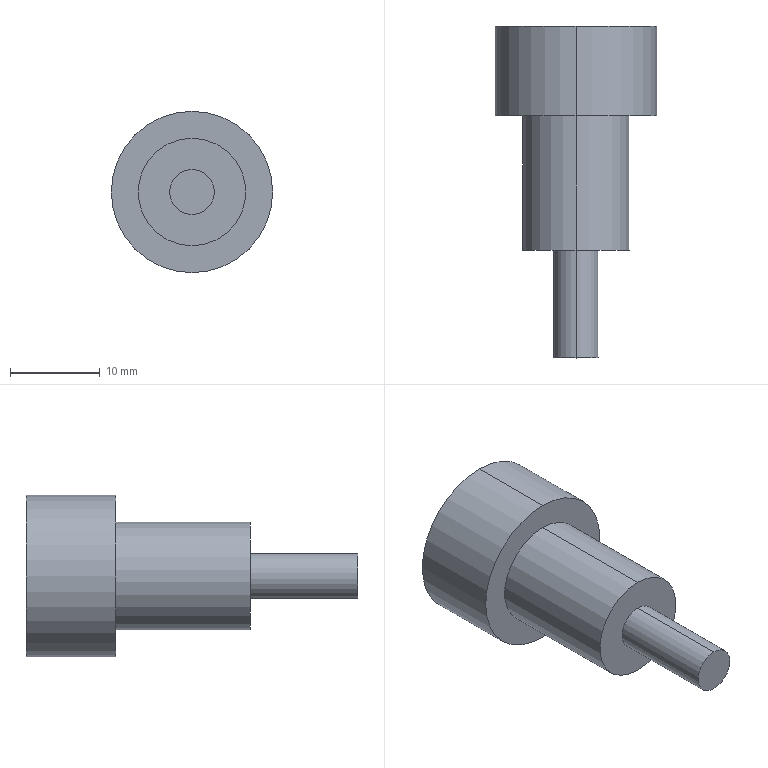Part | SolidWorks | features ICE 3, Extrusion 1 | 1 solid | 17 faces | box 18 x 37 x 18 mm | volume 4200 mm3 | plane 11 | cylinder 6 | commonest cylinder face diameters 5 x2 12 x2 18 x2
STEP:
#1=CARTESIAN_POINT('',(0.,37.,9.));
#2=VERTEX_POINT('',#1);
#3=CARTESIAN_POINT('',(0.,37.,-9.));
#4=VERTEX_POINT('',#3);
#5=CARTESIAN_POINT('',(0.,37.,0.));
#6=DIRECTION('',(0.,1.,0.));
#7=DIRECTION('',(0.,0.,1.));
#8=AXIS2_PLACEMENT_3D('',#5,#6,#7);
#9=CIRCLE('',#8,9.);
#10=EDGE_CURVE('',#2,#4,#9,.T.);
#11=ORIENTED_EDGE('',*,*,#10,.F.);
#12=CARTESIAN_POINT('',(0.,27.,9.));
#13=VERTEX_POINT('',#12);
#14=CARTESIAN_POINT('',(0.,37.,9.));
#15=DIRECTION('',(0.,-1.,0.));
#16=VECTOR('',#15,1000.);
#17=LINE('',#14,#16);
#18=EDGE_CURVE('',#2,#13,#17,.T.);
#19=ORIENTED_EDGE('',*,*,#18,.T.);
#20=CARTESIAN_POINT('',(0.,27.,-9.));
#21=VERTEX_POINT('',#20);
#22=CARTESIAN_POINT('',(0.,27.,0.));
#23=DIRECTION('',(0.,1.,0.));
#24=DIRECTION('',(0.,0.,1.));
#25=AXIS2_PLACEMENT_3D('',#22,#23,#24);
#26=CIRCLE('',#25,9.);
#27=EDGE_CURVE('',#13,#21,#26,.T.);
#28=ORIENTED_EDGE('',*,*,#27,.T.);
#29=CARTESIAN_POINT('',(0.,37.,-9.));
#30=DIRECTION('',(0.,-1.,0.));
#31=VECTOR('',#30,1000.);
#32=LINE('',#29,#31);
#33=EDGE_CURVE('',#4,#21,#32,.T.);
#34=ORIENTED_EDGE('',*,*,#33,.F.);
#35=EDGE_LOOP('',(#11,#19,#28,#34));
#36=FACE_OUTER_BOUND('',#35,.T.);
#37=CARTESIAN_POINT('',(0.,37.,0.));
#38=DIRECTION('',(0.,-1.,0.));
#39=DIRECTION('',(0.,0.,-1.));
#40=AXIS2_PLACEMENT_3D('',#37,#38,#39);
#41=CYLINDRICAL_SURFACE('',#40,9.);
#42=ADVANCED_FACE('',(#36),#41,.T.);
#43=CARTESIAN_POINT('',(0.,27.,6.));
#44=VERTEX_POINT('',#43);
#45=CARTESIAN_POINT('',(0.,27.,-6.));
#46=VERTEX_POINT('',#45);
#47=CARTESIAN_POINT('',(0.,27.,0.));
#48=DIRECTION('',(0.,1.,0.));
#49=DIRECTION('',(0.,0.,1.));
#50=AXIS2_PLACEMENT_3D('',#47,#48,#49);
#51=CIRCLE('',#50,6.);
#52=EDGE_CURVE('',#44,#46,#51,.T.);
#53=ORIENTED_EDGE('',*,*,#52,.F.);
#54=CARTESIAN_POINT('',(0.,12.,6.));
#55=VERTEX_POINT('',#54);
#56=CARTESIAN_POINT('',(0.,27.,6.));
#57=DIRECTION('',(0.,-1.,0.));
#58=VECTOR('',#57,1000.);
#59=LINE('',#56,#58);
#60=EDGE_CURVE('',#44,#55,#59,.T.);
#61=ORIENTED_EDGE('',*,*,#60,.T.);
#62=CARTESIAN_POINT('',(0.,12.,-6.));
#63=VERTEX_POINT('',#62);
#64=CARTESIAN_POINT('',(0.,12.,0.));
#65=DIRECTION('',(0.,1.,0.));
#66=DIRECTION('',(0.,0.,1.));
#67=AXIS2_PLACEMENT_3D('',#64,#65,#66);
#68=CIRCLE('',#67,6.);
#69=EDGE_CURVE('',#55,#63,#68,.T.);
#70=ORIENTED_EDGE('',*,*,#69,.T.);
#71=CARTESIAN_POINT('',(0.,27.,-6.));
#72=DIRECTION('',(0.,-1.,0.));
#73=VECTOR('',#72,1000.);
#74=LINE('',#71,#73);
#75=EDGE_CURVE('',#46,#63,#74,.T.);
#76=ORIENTED_EDGE('',*,*,#75,.F.);
#77=EDGE_LOOP('',(#53,#61,#70,#76));
#78=FACE_OUTER_BOUND('',#77,.T.);
#79=CARTESIAN_POINT('',(0.,27.,0.));
#80=DIRECTION('',(0.,-1.,0.));
#81=DIRECTION('',(0.,0.,-1.));
#82=AXIS2_PLACEMENT_3D('',#79,#80,#81);
#83=CYLINDRICAL_SURFACE('',#82,6.);
#84=ADVANCED_FACE('',(#78),#83,.T.);
#85=CARTESIAN_POINT('',(0.,12.,2.5));
#86=VERTEX_POINT('',#85);
#87=CARTESIAN_POINT('',(0.,12.,-2.5));
#88=VERTEX_POINT('',#87);
#89=CARTESIAN_POINT('',(0.,12.,0.));
#90=DIRECTION('',(0.,1.,0.));
#91=DIRECTION('',(0.,0.,1.));
#92=AXIS2_PLACEMENT_3D('',#89,#90,#91);
#93=CIRCLE('',#92,2.5);
#94=EDGE_CURVE('',#86,#88,#93,.T.);
#95=ORIENTED_EDGE('',*,*,#94,.F.);
#96=CARTESIAN_POINT('',(0.,0.,2.5));
#97=VERTEX_POINT('',#96);
#98=CARTESIAN_POINT('',(0.,12.,2.5));
#99=DIRECTION('',(0.,-1.,0.));
#100=VECTOR('',#99,1000.);
#101=LINE('',#98,#100);
#102=EDGE_CURVE('',#86,#97,#101,.T.);
#103=ORIENTED_EDGE('',*,*,#102,.T.);
#104=CARTESIAN_POINT('',(0.,0.,-2.5));
#105=VERTEX_POINT('',#104);
#106=CARTESIAN_POINT('',(0.,0.,0.));
#107=DIRECTION('',(0.,1.,0.));
#108=DIRECTION('',(0.,0.,1.));
#109=AXIS2_PLACEMENT_3D('',#106,#107,#108);
#110=CIRCLE('',#109,2.5);
#111=EDGE_CURVE('',#97,#105,#110,.T.);
#112=ORIENTED_EDGE('',*,*,#111,.T.);
#113=CARTESIAN_POINT('',(0.,12.,-2.5));
#114=DIRECTION('',(0.,-1.,0.));
#115=VECTOR('',#114,1000.);
#116=LINE('',#113,#115);
#117=EDGE_CURVE('',#88,#105,#116,.T.);
#118=ORIENTED_EDGE('',*,*,#117,.F.);
#119=EDGE_LOOP('',(#95,#103,#112,#118));
#120=FACE_OUTER_BOUND('',#119,.T.);
#121=CARTESIAN_POINT('',(0.,12.,0.));
#122=DIRECTION('',(0.,-1.,0.));
#123=DIRECTION('',(0.,0.,-1.));
#124=AXIS2_PLACEMENT_3D('',#121,#122,#123);
#125=CYLINDRICAL_SURFACE('',#124,2.5);
#126=ADVANCED_FACE('',(#120),#125,.T.);
#127=ORIENTED_EDGE('',*,*,#102,.F.);
#128=CARTESIAN_POINT('',(0.,12.,0.));
#129=DIRECTION('',(0.,1.,0.));
#130=DIRECTION('',(0.,0.,1.));
#131=AXIS2_PLACEMENT_3D('',#128,#129,#130);
#132=CIRCLE('',#131,2.5);
#133=EDGE_CURVE('',#88,#86,#132,.T.);
#134=ORIENTED_EDGE('',*,*,#133,.F.);
#135=ORIENTED_EDGE('',*,*,#117,.T.);
#136=CARTESIAN_POINT('',(0.,0.,0.));
#137=DIRECTION('',(0.,1.,0.));
#138=DIRECTION('',(0.,0.,1.));
#139=AXIS2_PLACEMENT_3D('',#136,#137,#138);
#140=CIRCLE('',#139,2.5);
#141=EDGE_CURVE('',#105,#97,#140,.T.);
#142=ORIENTED_EDGE('',*,*,#141,.T.);
#143=EDGE_LOOP('',(#127,#134,#135,#142));
#144=FACE_OUTER_BOUND('',#143,.T.);
#145=CARTESIAN_POINT('',(0.,12.,0.));
#146=DIRECTION('',(0.,-1.,0.));
#147=DIRECTION('',(0.,0.,-1.));
#148=AXIS2_PLACEMENT_3D('',#145,#146,#147);
#149=CYLINDRICAL_SURFACE('',#148,2.5);
#150=ADVANCED_FACE('',(#144),#149,.T.);
#151=ORIENTED_EDGE('',*,*,#141,.F.);
#152=ORIENTED_EDGE('',*,*,#111,.F.);
#153=EDGE_LOOP('',(#151,#152));
#154=FACE_OUTER_BOUND('',#153,.T.);
#155=CARTESIAN_POINT('',(0.,0.,0.));
#156=DIRECTION('',(0.,1.,0.));
#157=DIRECTION('',(0.,0.,1.));
#158=AXIS2_PLACEMENT_3D('',#155,#156,#157);
#159=PLANE('',#158);
#160=ADVANCED_FACE('',(#154),#159,.F.);
#161=ORIENTED_EDGE('',*,*,#60,.F.);
#162=CARTESIAN_POINT('',(0.,27.,0.));
#163=DIRECTION('',(0.,1.,0.));
#164=DIRECTION('',(0.,0.,1.));
#165=AXIS2_PLACEMENT_3D('',#162,#163,#164);
#166=CIRCLE('',#165,6.);
#167=EDGE_CURVE('',#46,#44,#166,.T.);
#168=ORIENTED_EDGE('',*,*,#167,.F.);
#169=ORIENTED_EDGE('',*,*,#75,.T.);
#170=CARTESIAN_POINT('',(0.,12.,0.));
#171=DIRECTION('',(0.,1.,0.));
#172=DIRECTION('',(0.,0.,1.));
#173=AXIS2_PLACEMENT_3D('',#170,#171,#172);
#174=CIRCLE('',#173,6.);
#175=EDGE_CURVE('',#63,#55,#174,.T.);
#176=ORIENTED_EDGE('',*,*,#175,.T.);
#177=EDGE_LOOP('',(#161,#168,#169,#176));
#178=FACE_OUTER_BOUND('',#177,.T.);
#179=CARTESIAN_POINT('',(0.,27.,0.));
#180=DIRECTION('',(0.,-1.,0.));
#181=DIRECTION('',(0.,0.,-1.));
#182=AXIS2_PLACEMENT_3D('',#179,#180,#181);
#183=CYLINDRICAL_SURFACE('',#182,6.);
#184=ADVANCED_FACE('',(#178),#183,.T.);
#185=ORIENTED_EDGE('',*,*,#133,.T.);
#186=ORIENTED_EDGE('',*,*,#94,.T.);
#187=EDGE_LOOP('',(#185,#186));
#188=FACE_BOUND('',#187,.T.);
#189=ORIENTED_EDGE('',*,*,#175,.F.);
#190=ORIENTED_EDGE('',*,*,#69,.F.);
#191=EDGE_LOOP('',(#189,#190));
#192=FACE_OUTER_BOUND('',#191,.T.);
#193=CARTESIAN_POINT('',(0.,12.,0.));
#194=DIRECTION('',(0.,1.,0.));
#195=DIRECTION('',(0.,0.,1.));
#196=AXIS2_PLACEMENT_3D('',#193,#194,#195);
#197=PLANE('',#196);
#198=ADVANCED_FACE('',(#188,#192),#197,.F.);
#199=ORIENTED_EDGE('',*,*,#18,.F.);
#200=CARTESIAN_POINT('',(0.,37.,0.));
#201=DIRECTION('',(0.,1.,0.));
#202=DIRECTION('',(0.,0.,1.));
#203=AXIS2_PLACEMENT_3D('',#200,#201,#202);
#204=CIRCLE('',#203,9.);
#205=EDGE_CURVE('',#4,#2,#204,.T.);
#206=ORIENTED_EDGE('',*,*,#205,.F.);
#207=ORIENTED_EDGE('',*,*,#33,.T.);
#208=CARTESIAN_POINT('',(0.,27.,0.));
#209=DIRECTION('',(0.,1.,0.));
#210=DIRECTION('',(0.,0.,1.));
#211=AXIS2_PLACEMENT_3D('',#208,#209,#210);
#212=CIRCLE('',#211,9.);
#213=EDGE_CURVE('',#21,#13,#212,.T.);
#214=ORIENTED_EDGE('',*,*,#213,.T.);
#215=EDGE_LOOP('',(#199,#206,#207,#214));
#216=FACE_OUTER_BOUND('',#215,.T.);
#217=CARTESIAN_POINT('',(0.,37.,0.));
#218=DIRECTION('',(0.,-1.,0.));
#219=DIRECTION('',(0.,0.,-1.));
#220=AXIS2_PLACEMENT_3D('',#217,#218,#219);
#221=CYLINDRICAL_SURFACE('',#220,9.);
#222=ADVANCED_FACE('',(#216),#221,.T.);
#223=CARTESIAN_POINT('',(4.,37.,-2.309));
#224=VERTEX_POINT('',#223);
#225=CARTESIAN_POINT('',(0.,37.,-4.619));
#226=VERTEX_POINT('',#225);
#227=CARTESIAN_POINT('',(4.,37.,-2.309));
#228=DIRECTION('',(-0.866,0.,-0.5));
#229=VECTOR('',#228,1000.);
#230=LINE('',#227,#229);
#231=EDGE_CURVE('',#224,#226,#230,.T.);
#232=ORIENTED_EDGE('',*,*,#231,.F.);
#233=CARTESIAN_POINT('',(4.,37.,2.309));
#234=VERTEX_POINT('',#233);
#235=CARTESIAN_POINT('',(4.,37.,2.309));
#236=DIRECTION('',(0.,0.,-1.));
#237=VECTOR('',#236,1000.);
#238=LINE('',#235,#237);
#239=EDGE_CURVE('',#234,#224,#238,.T.);
#240=ORIENTED_EDGE('',*,*,#239,.F.);
#241=CARTESIAN_POINT('',(0.,37.,4.619));
#242=VERTEX_POINT('',#241);
#243=CARTESIAN_POINT('',(0.,37.,4.619));
#244=DIRECTION('',(0.866,0.,-0.5));
#245=VECTOR('',#244,1000.);
#246=LINE('',#243,#245);
#247=EDGE_CURVE('',#242,#234,#246,.T.);
#248=ORIENTED_EDGE('',*,*,#247,.F.);
#249=CARTESIAN_POINT('',(-4.,37.,2.309));
#250=VERTEX_POINT('',#249);
#251=CARTESIAN_POINT('',(-4.,37.,2.309));
#252=DIRECTION('',(0.866,0.,0.5));
#253=VECTOR('',#252,1000.);
#254=LINE('',#251,#253);
#255=EDGE_CURVE('',#250,#242,#254,.T.);
#256=ORIENTED_EDGE('',*,*,#255,.F.);
#257=CARTESIAN_POINT('',(-4.,37.,-2.309));
#258=VERTEX_POINT('',#257);
#259=CARTESIAN_POINT('',(-4.,37.,-2.309));
#260=DIRECTION('',(0.,0.,1.));
#261=VECTOR('',#260,1000.);
#262=LINE('',#259,#261);
#263=EDGE_CURVE('',#258,#250,#262,.T.);
#264=ORIENTED_EDGE('',*,*,#263,.F.);
#265=CARTESIAN_POINT('',(0.,37.,-4.619));
#266=DIRECTION('',(-0.866,0.,0.5));
#267=VECTOR('',#266,1000.);
#268=LINE('',#265,#267);
#269=EDGE_CURVE('',#226,#258,#268,.T.);
#270=ORIENTED_EDGE('',*,*,#269,.F.);
#271=EDGE_LOOP('',(#232,#240,#248,#256,#264,#270));
#272=FACE_BOUND('',#271,.T.);
#273=ORIENTED_EDGE('',*,*,#205,.T.);
#274=ORIENTED_EDGE('',*,*,#10,.T.);
#275=EDGE_LOOP('',(#273,#274));
#276=FACE_OUTER_BOUND('',#275,.T.);
#277=CARTESIAN_POINT('',(0.,37.,0.));
#278=DIRECTION('',(0.,1.,0.));
#279=DIRECTION('',(0.,0.,1.));
#280=AXIS2_PLACEMENT_3D('',#277,#278,#279);
#281=PLANE('',#280);
#282=ADVANCED_FACE('',(#272,#276),#281,.T.);
#283=ORIENTED_EDGE('',*,*,#167,.T.);
#284=ORIENTED_EDGE('',*,*,#52,.T.);
#285=EDGE_LOOP('',(#283,#284));
#286=FACE_BOUND('',#285,.T.);
#287=ORIENTED_EDGE('',*,*,#213,.F.);
#288=ORIENTED_EDGE('',*,*,#27,.F.);
#289=EDGE_LOOP('',(#287,#288));
#290=FACE_OUTER_BOUND('',#289,.T.);
#291=CARTESIAN_POINT('',(0.,27.,0.));
#292=DIRECTION('',(0.,1.,0.));
#293=DIRECTION('',(0.,0.,1.));
#294=AXIS2_PLACEMENT_3D('',#291,#292,#293);
#295=PLANE('',#294);
#296=ADVANCED_FACE('',(#286,#290),#295,.F.);
#297=ORIENTED_EDGE('',*,*,#231,.T.);
#298=CARTESIAN_POINT('',(0.,32.,-4.619));
#299=VERTEX_POINT('',#298);
#300=CARTESIAN_POINT('',(0.,32.,-4.619));
#301=DIRECTION('',(0.,1.,0.));
#302=VECTOR('',#301,1000.);
#303=LINE('',#300,#302);
#304=EDGE_CURVE('',#299,#226,#303,.T.);
#305=ORIENTED_EDGE('',*,*,#304,.F.);
#306=CARTESIAN_POINT('',(4.,32.,-2.309));
#307=VERTEX_POINT('',#306);
#308=CARTESIAN_POINT('',(4.,32.,-2.309));
#309=DIRECTION('',(-0.866,0.,-0.5));
#310=VECTOR('',#309,1000.);
#311=LINE('',#308,#310);
#312=EDGE_CURVE('',#307,#299,#311,.T.);
#313=ORIENTED_EDGE('',*,*,#312,.F.);
#314=CARTESIAN_POINT('',(4.,32.,-2.309));
#315=DIRECTION('',(0.,1.,0.));
#316=VECTOR('',#315,1000.);
#317=LINE('',#314,#316);
#318=EDGE_CURVE('',#307,#224,#317,.T.);
#319=ORIENTED_EDGE('',*,*,#318,.T.);
#320=EDGE_LOOP('',(#297,#305,#313,#319));
#321=FACE_OUTER_BOUND('',#320,.T.);
#322=CARTESIAN_POINT('',(4.,32.,-2.309));
#323=DIRECTION('',(0.5,0.,-0.866));
#324=DIRECTION('',(-0.866,0.,-0.5));
#325=AXIS2_PLACEMENT_3D('',#322,#323,#324);
#326=PLANE('',#325);
#327=ADVANCED_FACE('',(#321),#326,.F.);
#328=ORIENTED_EDGE('',*,*,#239,.T.);
#329=ORIENTED_EDGE('',*,*,#318,.F.);
#330=CARTESIAN_POINT('',(4.,32.,2.309));
#331=VERTEX_POINT('',#330);
#332=CARTESIAN_POINT('',(4.,32.,2.309));
#333=DIRECTION('',(0.,0.,-1.));
#334=VECTOR('',#333,1000.);
#335=LINE('',#332,#334);
#336=EDGE_CURVE('',#331,#307,#335,.T.);
#337=ORIENTED_EDGE('',*,*,#336,.F.);
#338=CARTESIAN_POINT('',(4.,32.,2.309));
#339=DIRECTION('',(0.,1.,0.));
#340=VECTOR('',#339,1000.);
#341=LINE('',#338,#340);
#342=EDGE_CURVE('',#331,#234,#341,.T.);
#343=ORIENTED_EDGE('',*,*,#342,.T.);
#344=EDGE_LOOP('',(#328,#329,#337,#343));
#345=FACE_OUTER_BOUND('',#344,.T.);
#346=CARTESIAN_POINT('',(4.,32.,2.309));
#347=DIRECTION('',(1.,0.,0.));
#348=DIRECTION('',(0.,0.,-1.));
#349=AXIS2_PLACEMENT_3D('',#346,#347,#348);
#350=PLANE('',#349);
#351=ADVANCED_FACE('',(#345),#350,.F.);
#352=ORIENTED_EDGE('',*,*,#247,.T.);
#353=ORIENTED_EDGE('',*,*,#342,.F.);
#354=CARTESIAN_POINT('',(0.,32.,4.619));
#355=VERTEX_POINT('',#354);
#356=CARTESIAN_POINT('',(0.,32.,4.619));
#357=DIRECTION('',(0.866,0.,-0.5));
#358=VECTOR('',#357,1000.);
#359=LINE('',#356,#358);
#360=EDGE_CURVE('',#355,#331,#359,.T.);
#361=ORIENTED_EDGE('',*,*,#360,.F.);
#362=CARTESIAN_POINT('',(0.,32.,4.619));
#363=DIRECTION('',(0.,1.,0.));
#364=VECTOR('',#363,1000.);
#365=LINE('',#362,#364);
#366=EDGE_CURVE('',#355,#242,#365,.T.);
#367=ORIENTED_EDGE('',*,*,#366,.T.);
#368=EDGE_LOOP('',(#352,#353,#361,#367));
#369=FACE_OUTER_BOUND('',#368,.T.);
#370=CARTESIAN_POINT('',(0.,32.,4.619));
#371=DIRECTION('',(0.5,0.,0.866));
#372=DIRECTION('',(0.866,0.,-0.5));
#373=AXIS2_PLACEMENT_3D('',#370,#371,#372);
#374=PLANE('',#373);
#375=ADVANCED_FACE('',(#369),#374,.F.);
#376=ORIENTED_EDGE('',*,*,#255,.T.);
#377=ORIENTED_EDGE('',*,*,#366,.F.);
#378=CARTESIAN_POINT('',(-4.,32.,2.309));
#379=VERTEX_POINT('',#378);
#380=CARTESIAN_POINT('',(-4.,32.,2.309));
#381=DIRECTION('',(0.866,0.,0.5));
#382=VECTOR('',#381,1000.);
#383=LINE('',#380,#382);
#384=EDGE_CURVE('',#379,#355,#383,.T.);
#385=ORIENTED_EDGE('',*,*,#384,.F.);
#386=CARTESIAN_POINT('',(-4.,32.,2.309));
#387=DIRECTION('',(0.,1.,0.));
#388=VECTOR('',#387,1000.);
#389=LINE('',#386,#388);
#390=EDGE_CURVE('',#379,#250,#389,.T.);
#391=ORIENTED_EDGE('',*,*,#390,.T.);
#392=EDGE_LOOP('',(#376,#377,#385,#391));
#393=FACE_OUTER_BOUND('',#392,.T.);
#394=CARTESIAN_POINT('',(-4.,32.,2.309));
#395=DIRECTION('',(-0.5,0.,0.866));
#396=DIRECTION('',(0.866,0.,0.5));
#397=AXIS2_PLACEMENT_3D('',#394,#395,#396);
#398=PLANE('',#397);
#399=ADVANCED_FACE('',(#393),#398,.F.);
#400=ORIENTED_EDGE('',*,*,#263,.T.);
#401=ORIENTED_EDGE('',*,*,#390,.F.);
#402=CARTESIAN_POINT('',(-4.,32.,-2.309));
#403=VERTEX_POINT('',#402);
#404=CARTESIAN_POINT('',(-4.,32.,-2.309));
#405=DIRECTION('',(0.,0.,1.));
#406=VECTOR('',#405,1000.);
#407=LINE('',#404,#406);
#408=EDGE_CURVE('',#403,#379,#407,.T.);
#409=ORIENTED_EDGE('',*,*,#408,.F.);
#410=CARTESIAN_POINT('',(-4.,32.,-2.309));
#411=DIRECTION('',(0.,1.,0.));
#412=VECTOR('',#411,1000.);
#413=LINE('',#410,#412);
#414=EDGE_CURVE('',#403,#258,#413,.T.);
#415=ORIENTED_EDGE('',*,*,#414,.T.);
#416=EDGE_LOOP('',(#400,#401,#409,#415));
#417=FACE_OUTER_BOUND('',#416,.T.);
#418=CARTESIAN_POINT('',(-4.,32.,-2.309));
#419=DIRECTION('',(-1.,0.,0.));
#420=DIRECTION('',(0.,0.,1.));
#421=AXIS2_PLACEMENT_3D('',#418,#419,#420);
#422=PLANE('',#421);
#423=ADVANCED_FACE('',(#417),#422,.F.);
#424=ORIENTED_EDGE('',*,*,#269,.T.);
#425=ORIENTED_EDGE('',*,*,#414,.F.);
#426=CARTESIAN_POINT('',(0.,32.,-4.619));
#427=DIRECTION('',(-0.866,0.,0.5));
#428=VECTOR('',#427,1000.);
#429=LINE('',#426,#428);
#430=EDGE_CURVE('',#299,#403,#429,.T.);
#431=ORIENTED_EDGE('',*,*,#430,.F.);
#432=ORIENTED_EDGE('',*,*,#304,.T.);
#433=EDGE_LOOP('',(#424,#425,#431,#432));
#434=FACE_OUTER_BOUND('',#433,.T.);
#435=CARTESIAN_POINT('',(0.,32.,-4.619));
#436=DIRECTION('',(-0.5,0.,-0.866));
#437=DIRECTION('',(-0.866,0.,0.5));
#438=AXIS2_PLACEMENT_3D('',#435,#436,#437);
#439=PLANE('',#438);
#440=ADVANCED_FACE('',(#434),#439,.F.);
#441=ORIENTED_EDGE('',*,*,#312,.T.);
#442=ORIENTED_EDGE('',*,*,#430,.T.);
#443=ORIENTED_EDGE('',*,*,#408,.T.);
#444=ORIENTED_EDGE('',*,*,#384,.T.);
#445=ORIENTED_EDGE('',*,*,#360,.T.);
#446=ORIENTED_EDGE('',*,*,#336,.T.);
#447=EDGE_LOOP('',(#441,#442,#443,#444,#445,#446));
#448=FACE_OUTER_BOUND('',#447,.T.);
#449=CARTESIAN_POINT('',(0.,32.,0.));
#450=DIRECTION('',(0.,1.,0.));
#451=DIRECTION('',(0.,0.,1.));
#452=AXIS2_PLACEMENT_3D('',#449,#450,#451);
#453=PLANE('',#452);
#454=ADVANCED_FACE('',(#448),#453,.T.);
#455=CLOSED_SHELL('',(#42,#84,#126,#150,#160,#184,#198,#222,#282,#296,#327,#351,#375,#399,#423,#440,#454));
#456=MANIFOLD_SOLID_BREP('',#455);
#457=CARTESIAN_POINT('',(0.,0.,0.));
#458=DIRECTION('',(0.,0.,1.));
#459=DIRECTION('',(1.,0.,0.));
#460=AXIS2_PLACEMENT_3D('',#457,#458,#459);
#461=(LENGTH_UNIT()NAMED_UNIT(*)SI_UNIT(.MILLI.,.METRE.));
#462=UNCERTAINTY_MEASURE_WITH_UNIT(LENGTH_MEASURE(0.00001),#461,'','');
#463=(NAMED_UNIT(*)PLANE_ANGLE_UNIT()SI_UNIT($,.RADIAN.));
#464=(NAMED_UNIT(*)SI_UNIT($,.STERADIAN.)SOLID_ANGLE_UNIT());
#465=(GEOMETRIC_REPRESENTATION_CONTEXT(3)GLOBAL_UNCERTAINTY_ASSIGNED_CONTEXT((#462))GLOBAL_UNIT_ASSIGNED_CONTEXT((#461,#463,#464))REPRESENTATION_CONTEXT('',''));
#466=ADVANCED_BREP_SHAPE_REPRESENTATION('',(#456,#460),#465);